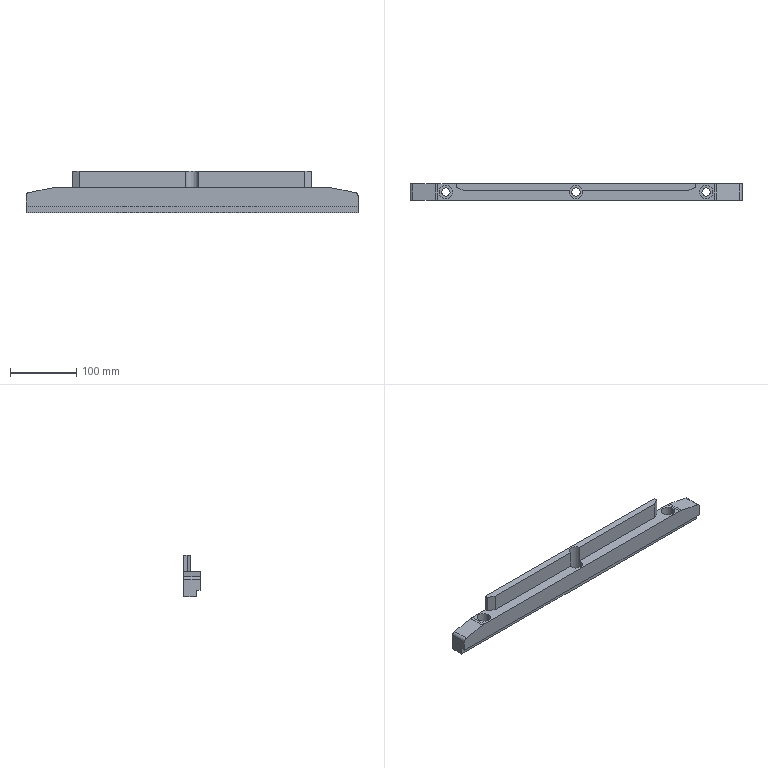Part | 1 solid | 60 faces | box 500 x 25 x 62.5 mm | volume 435147 mm3 | cylinder 32 | plane 28 | commonest cylinder face diameters 17 x16 12.5 x6 20 x6 10 x2 40 x2